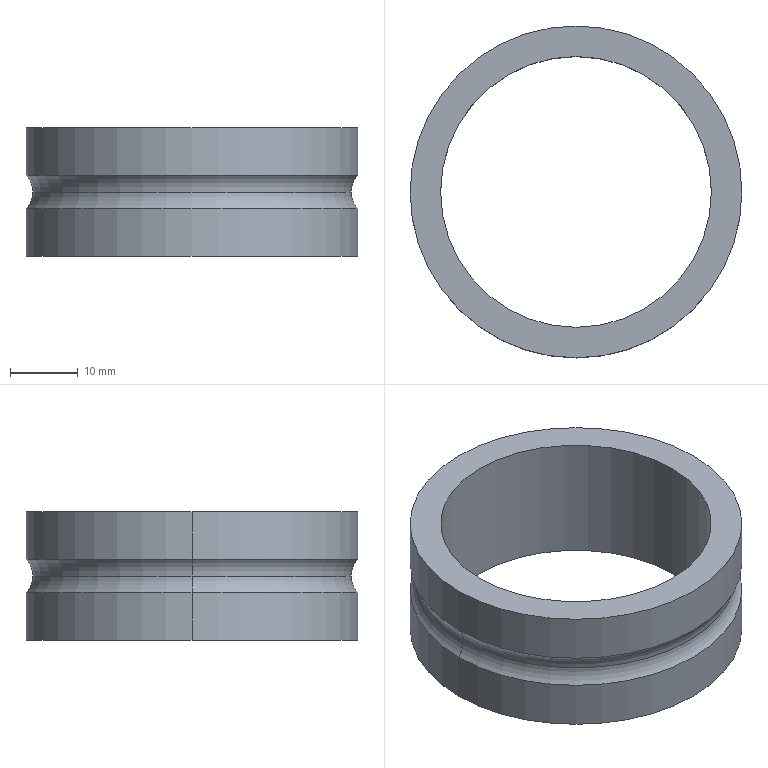Part | SolidWorks | 1 solid | 12 faces | box 49 x 49 x 19 mm | volume 11442 mm3 | cylinder 6 | torus 4 | plane 2 | commonest cylinder face diameters 49 x4 40 x2
STEP:
#1=CARTESIAN_POINT('',(-23.5,0.,-9.5));
#2=VERTEX_POINT('',#1);
#3=CARTESIAN_POINT('',(-24.5,0.,-11.949));
#4=VERTEX_POINT('',#3);
#5=CARTESIAN_POINT('',(-27.,0.,-9.5));
#6=DIRECTION('',(0.,1.,0.));
#7=DIRECTION('',(1.,0.,0.));
#8=AXIS2_PLACEMENT_3D('',#5,#6,#7);
#9=CIRCLE('',#8,3.5);
#10=EDGE_CURVE('',#2,#4,#9,.T.);
#11=ORIENTED_EDGE('',*,*,#10,.T.);
#12=CARTESIAN_POINT('',(24.5,0.,-11.949));
#13=VERTEX_POINT('',#12);
#14=CARTESIAN_POINT('',(0.,0.,-11.949));
#15=DIRECTION('',(0.,0.,-1.));
#16=DIRECTION('',(1.,0.,0.));
#17=AXIS2_PLACEMENT_3D('',#14,#15,#16);
#18=CIRCLE('',#17,24.5);
#19=EDGE_CURVE('',#13,#4,#18,.T.);
#20=ORIENTED_EDGE('',*,*,#19,.F.);
#21=CARTESIAN_POINT('',(23.5,0.,-9.5));
#22=VERTEX_POINT('',#21);
#23=CARTESIAN_POINT('',(27.,0.,-9.5));
#24=DIRECTION('',(0.,-1.,0.));
#25=DIRECTION('',(-1.,0.,0.));
#26=AXIS2_PLACEMENT_3D('',#23,#24,#25);
#27=CIRCLE('',#26,3.5);
#28=EDGE_CURVE('',#22,#13,#27,.T.);
#29=ORIENTED_EDGE('',*,*,#28,.F.);
#30=CARTESIAN_POINT('',(0.,0.,-9.5));
#31=DIRECTION('',(0.,0.,-1.));
#32=DIRECTION('',(1.,0.,0.));
#33=AXIS2_PLACEMENT_3D('',#30,#31,#32);
#34=CIRCLE('',#33,23.5);
#35=EDGE_CURVE('',#22,#2,#34,.T.);
#36=ORIENTED_EDGE('',*,*,#35,.T.);
#37=EDGE_LOOP('',(#11,#20,#29,#36));
#38=FACE_OUTER_BOUND('',#37,.T.);
#39=CARTESIAN_POINT('',(0.,0.,-9.5));
#40=DIRECTION('',(0.,0.,1.));
#41=DIRECTION('',(-1.,0.,0.));
#42=AXIS2_PLACEMENT_3D('',#39,#40,#41);
#43=TOROIDAL_SURFACE('',#42,27.,3.5);
#44=ADVANCED_FACE('',(#38),#43,.F.);
#45=ORIENTED_EDGE('',*,*,#28,.T.);
#46=CARTESIAN_POINT('',(0.,0.,-11.949));
#47=DIRECTION('',(0.,0.,-1.));
#48=DIRECTION('',(-1.,0.,0.));
#49=AXIS2_PLACEMENT_3D('',#46,#47,#48);
#50=CIRCLE('',#49,24.5);
#51=EDGE_CURVE('',#4,#13,#50,.T.);
#52=ORIENTED_EDGE('',*,*,#51,.F.);
#53=ORIENTED_EDGE('',*,*,#10,.F.);
#54=CARTESIAN_POINT('',(0.,0.,-9.5));
#55=DIRECTION('',(0.,0.,-1.));
#56=DIRECTION('',(-1.,0.,0.));
#57=AXIS2_PLACEMENT_3D('',#54,#55,#56);
#58=CIRCLE('',#57,23.5);
#59=EDGE_CURVE('',#2,#22,#58,.T.);
#60=ORIENTED_EDGE('',*,*,#59,.T.);
#61=EDGE_LOOP('',(#45,#52,#53,#60));
#62=FACE_OUTER_BOUND('',#61,.T.);
#63=CARTESIAN_POINT('',(0.,0.,-9.5));
#64=DIRECTION('',(0.,0.,1.));
#65=DIRECTION('',(1.,0.,0.));
#66=AXIS2_PLACEMENT_3D('',#63,#64,#65);
#67=TOROIDAL_SURFACE('',#66,27.,3.5);
#68=ADVANCED_FACE('',(#62),#67,.F.);
#69=CARTESIAN_POINT('',(-24.5,0.,0.));
#70=VERTEX_POINT('',#69);
#71=CARTESIAN_POINT('',(24.5,0.,0.));
#72=VERTEX_POINT('',#71);
#73=CARTESIAN_POINT('',(0.,0.,0.));
#74=DIRECTION('',(0.,0.,-1.));
#75=DIRECTION('',(-1.,0.,0.));
#76=AXIS2_PLACEMENT_3D('',#73,#74,#75);
#77=CIRCLE('',#76,24.5);
#78=EDGE_CURVE('',#70,#72,#77,.T.);
#79=ORIENTED_EDGE('',*,*,#78,.T.);
#80=CARTESIAN_POINT('',(24.5,0.,-7.051));
#81=VERTEX_POINT('',#80);
#82=CARTESIAN_POINT('',(24.5,0.,0.));
#83=DIRECTION('',(0.,0.,-1.));
#84=VECTOR('',#83,1000.);
#85=LINE('',#82,#84);
#86=EDGE_CURVE('',#72,#81,#85,.T.);
#87=ORIENTED_EDGE('',*,*,#86,.T.);
#88=CARTESIAN_POINT('',(-24.5,0.,-7.051));
#89=VERTEX_POINT('',#88);
#90=CARTESIAN_POINT('',(0.,0.,-7.051));
#91=DIRECTION('',(0.,0.,1.));
#92=DIRECTION('',(1.,0.,0.));
#93=AXIS2_PLACEMENT_3D('',#90,#91,#92);
#94=CIRCLE('',#93,24.5);
#95=EDGE_CURVE('',#81,#89,#94,.T.);
#96=ORIENTED_EDGE('',*,*,#95,.T.);
#97=CARTESIAN_POINT('',(-24.5,0.,0.));
#98=DIRECTION('',(0.,0.,-1.));
#99=VECTOR('',#98,1000.);
#100=LINE('',#97,#99);
#101=EDGE_CURVE('',#70,#89,#100,.T.);
#102=ORIENTED_EDGE('',*,*,#101,.F.);
#103=EDGE_LOOP('',(#79,#87,#96,#102));
#104=FACE_OUTER_BOUND('',#103,.T.);
#105=CARTESIAN_POINT('',(0.,0.,0.));
#106=DIRECTION('',(0.,0.,1.));
#107=DIRECTION('',(1.,0.,0.));
#108=AXIS2_PLACEMENT_3D('',#105,#106,#107);
#109=CYLINDRICAL_SURFACE('',#108,24.5);
#110=ADVANCED_FACE('',(#104),#109,.T.);
#111=ORIENTED_EDGE('',*,*,#59,.F.);
#112=CARTESIAN_POINT('',(-27.,0.,-9.5));
#113=DIRECTION('',(0.,1.,0.));
#114=DIRECTION('',(0.7143,0.,0.6999));
#115=AXIS2_PLACEMENT_3D('',#112,#113,#114);
#116=CIRCLE('',#115,3.5);
#117=EDGE_CURVE('',#89,#2,#116,.T.);
#118=ORIENTED_EDGE('',*,*,#117,.F.);
#119=ORIENTED_EDGE('',*,*,#95,.F.);
#120=CARTESIAN_POINT('',(27.,0.,-9.5));
#121=DIRECTION('',(0.,-1.,0.));
#122=DIRECTION('',(-0.7143,0.,0.6999));
#123=AXIS2_PLACEMENT_3D('',#120,#121,#122);
#124=CIRCLE('',#123,3.5);
#125=EDGE_CURVE('',#81,#22,#124,.T.);
#126=ORIENTED_EDGE('',*,*,#125,.T.);
#127=EDGE_LOOP('',(#111,#118,#119,#126));
#128=FACE_OUTER_BOUND('',#127,.T.);
#129=CARTESIAN_POINT('',(0.,0.,-9.5));
#130=DIRECTION('',(0.,0.,1.));
#131=DIRECTION('',(1.,0.,0.));
#132=AXIS2_PLACEMENT_3D('',#129,#130,#131);
#133=TOROIDAL_SURFACE('',#132,27.,3.5);
#134=ADVANCED_FACE('',(#128),#133,.F.);
#135=ORIENTED_EDGE('',*,*,#35,.F.);
#136=ORIENTED_EDGE('',*,*,#125,.F.);
#137=CARTESIAN_POINT('',(0.,0.,-7.051));
#138=DIRECTION('',(0.,0.,1.));
#139=DIRECTION('',(-1.,0.,0.));
#140=AXIS2_PLACEMENT_3D('',#137,#138,#139);
#141=CIRCLE('',#140,24.5);
#142=EDGE_CURVE('',#89,#81,#141,.T.);
#143=ORIENTED_EDGE('',*,*,#142,.F.);
#144=ORIENTED_EDGE('',*,*,#117,.T.);
#145=EDGE_LOOP('',(#135,#136,#143,#144));
#146=FACE_OUTER_BOUND('',#145,.T.);
#147=CARTESIAN_POINT('',(0.,0.,-9.5));
#148=DIRECTION('',(0.,0.,1.));
#149=DIRECTION('',(-1.,0.,0.));
#150=AXIS2_PLACEMENT_3D('',#147,#148,#149);
#151=TOROIDAL_SURFACE('',#150,27.,3.5);
#152=ADVANCED_FACE('',(#146),#151,.F.);
#153=ORIENTED_EDGE('',*,*,#86,.F.);
#154=CARTESIAN_POINT('',(0.,0.,0.));
#155=DIRECTION('',(0.,0.,-1.));
#156=DIRECTION('',(1.,0.,0.));
#157=AXIS2_PLACEMENT_3D('',#154,#155,#156);
#158=CIRCLE('',#157,24.5);
#159=EDGE_CURVE('',#72,#70,#158,.T.);
#160=ORIENTED_EDGE('',*,*,#159,.T.);
#161=ORIENTED_EDGE('',*,*,#101,.T.);
#162=ORIENTED_EDGE('',*,*,#142,.T.);
#163=EDGE_LOOP('',(#153,#160,#161,#162));
#164=FACE_OUTER_BOUND('',#163,.T.);
#165=CARTESIAN_POINT('',(0.,0.,0.));
#166=DIRECTION('',(0.,0.,1.));
#167=DIRECTION('',(1.,0.,0.));
#168=AXIS2_PLACEMENT_3D('',#165,#166,#167);
#169=CYLINDRICAL_SURFACE('',#168,24.5);
#170=ADVANCED_FACE('',(#164),#169,.T.);
#171=CARTESIAN_POINT('',(-20.,0.,0.));
#172=VERTEX_POINT('',#171);
#173=CARTESIAN_POINT('',(20.,0.,0.));
#174=VERTEX_POINT('',#173);
#175=CARTESIAN_POINT('',(0.,0.,0.));
#176=DIRECTION('',(0.,0.,1.));
#177=DIRECTION('',(-1.,0.,0.));
#178=AXIS2_PLACEMENT_3D('',#175,#176,#177);
#179=CIRCLE('',#178,20.);
#180=EDGE_CURVE('',#172,#174,#179,.T.);
#181=ORIENTED_EDGE('',*,*,#180,.F.);
#182=CARTESIAN_POINT('',(0.,0.,0.));
#183=DIRECTION('',(0.,0.,1.));
#184=DIRECTION('',(1.,0.,0.));
#185=AXIS2_PLACEMENT_3D('',#182,#183,#184);
#186=CIRCLE('',#185,20.);
#187=EDGE_CURVE('',#174,#172,#186,.T.);
#188=ORIENTED_EDGE('',*,*,#187,.F.);
#189=EDGE_LOOP('',(#181,#188));
#190=FACE_BOUND('',#189,.T.);
#191=ORIENTED_EDGE('',*,*,#78,.F.);
#192=ORIENTED_EDGE('',*,*,#159,.F.);
#193=EDGE_LOOP('',(#191,#192));
#194=FACE_OUTER_BOUND('',#193,.T.);
#195=CARTESIAN_POINT('',(0.,-20.,0.));
#196=DIRECTION('',(0.,0.,1.));
#197=DIRECTION('',(1.,0.,0.));
#198=AXIS2_PLACEMENT_3D('',#195,#196,#197);
#199=PLANE('',#198);
#200=ADVANCED_FACE('',(#190,#194),#199,.T.);
#201=CARTESIAN_POINT('',(20.,0.,-19.));
#202=VERTEX_POINT('',#201);
#203=CARTESIAN_POINT('',(20.,0.,0.));
#204=DIRECTION('',(0.,0.,-1.));
#205=VECTOR('',#204,1000.);
#206=LINE('',#203,#205);
#207=EDGE_CURVE('',#174,#202,#206,.T.);
#208=ORIENTED_EDGE('',*,*,#207,.F.);
#209=ORIENTED_EDGE('',*,*,#187,.T.);
#210=CARTESIAN_POINT('',(-20.,0.,-19.));
#211=VERTEX_POINT('',#210);
#212=CARTESIAN_POINT('',(-20.,0.,0.));
#213=DIRECTION('',(0.,0.,-1.));
#214=VECTOR('',#213,1000.);
#215=LINE('',#212,#214);
#216=EDGE_CURVE('',#172,#211,#215,.T.);
#217=ORIENTED_EDGE('',*,*,#216,.T.);
#218=CARTESIAN_POINT('',(0.,0.,-19.));
#219=DIRECTION('',(0.,0.,-1.));
#220=DIRECTION('',(-1.,0.,0.));
#221=AXIS2_PLACEMENT_3D('',#218,#219,#220);
#222=CIRCLE('',#221,20.);
#223=EDGE_CURVE('',#211,#202,#222,.T.);
#224=ORIENTED_EDGE('',*,*,#223,.T.);
#225=EDGE_LOOP('',(#208,#209,#217,#224));
#226=FACE_OUTER_BOUND('',#225,.T.);
#227=CARTESIAN_POINT('',(0.,0.,0.));
#228=DIRECTION('',(0.,0.,1.));
#229=DIRECTION('',(1.,0.,0.));
#230=AXIS2_PLACEMENT_3D('',#227,#228,#229);
#231=CYLINDRICAL_SURFACE('',#230,20.);
#232=ADVANCED_FACE('',(#226),#231,.F.);
#233=ORIENTED_EDGE('',*,*,#180,.T.);
#234=ORIENTED_EDGE('',*,*,#207,.T.);
#235=CARTESIAN_POINT('',(0.,0.,-19.));
#236=DIRECTION('',(0.,0.,-1.));
#237=DIRECTION('',(1.,0.,0.));
#238=AXIS2_PLACEMENT_3D('',#235,#236,#237);
#239=CIRCLE('',#238,20.);
#240=EDGE_CURVE('',#202,#211,#239,.T.);
#241=ORIENTED_EDGE('',*,*,#240,.T.);
#242=ORIENTED_EDGE('',*,*,#216,.F.);
#243=EDGE_LOOP('',(#233,#234,#241,#242));
#244=FACE_OUTER_BOUND('',#243,.T.);
#245=CARTESIAN_POINT('',(0.,0.,0.));
#246=DIRECTION('',(0.,0.,1.));
#247=DIRECTION('',(1.,0.,0.));
#248=AXIS2_PLACEMENT_3D('',#245,#246,#247);
#249=CYLINDRICAL_SURFACE('',#248,20.);
#250=ADVANCED_FACE('',(#244),#249,.F.);
#251=ORIENTED_EDGE('',*,*,#223,.F.);
#252=ORIENTED_EDGE('',*,*,#240,.F.);
#253=EDGE_LOOP('',(#251,#252));
#254=FACE_BOUND('',#253,.T.);
#255=CARTESIAN_POINT('',(-24.5,0.,-19.));
#256=VERTEX_POINT('',#255);
#257=CARTESIAN_POINT('',(24.5,0.,-19.));
#258=VERTEX_POINT('',#257);
#259=CARTESIAN_POINT('',(0.,0.,-19.));
#260=DIRECTION('',(0.,0.,1.));
#261=DIRECTION('',(-1.,0.,0.));
#262=AXIS2_PLACEMENT_3D('',#259,#260,#261);
#263=CIRCLE('',#262,24.5);
#264=EDGE_CURVE('',#256,#258,#263,.T.);
#265=ORIENTED_EDGE('',*,*,#264,.F.);
#266=CARTESIAN_POINT('',(0.,0.,-19.));
#267=DIRECTION('',(0.,0.,1.));
#268=DIRECTION('',(1.,0.,0.));
#269=AXIS2_PLACEMENT_3D('',#266,#267,#268);
#270=CIRCLE('',#269,24.5);
#271=EDGE_CURVE('',#258,#256,#270,.T.);
#272=ORIENTED_EDGE('',*,*,#271,.F.);
#273=EDGE_LOOP('',(#265,#272));
#274=FACE_OUTER_BOUND('',#273,.T.);
#275=CARTESIAN_POINT('',(0.,-24.5,-19.));
#276=DIRECTION('',(0.,0.,-1.));
#277=DIRECTION('',(0.,-1.,0.));
#278=AXIS2_PLACEMENT_3D('',#275,#276,#277);
#279=PLANE('',#278);
#280=ADVANCED_FACE('',(#254,#274),#279,.T.);
#281=CARTESIAN_POINT('',(24.5,0.,-11.949));
#282=DIRECTION('',(0.,0.,-1.));
#283=VECTOR('',#282,1000.);
#284=LINE('',#281,#283);
#285=EDGE_CURVE('',#13,#258,#284,.T.);
#286=ORIENTED_EDGE('',*,*,#285,.F.);
#287=ORIENTED_EDGE('',*,*,#19,.T.);
#288=CARTESIAN_POINT('',(-24.5,0.,-11.949));
#289=DIRECTION('',(0.,0.,-1.));
#290=VECTOR('',#289,1000.);
#291=LINE('',#288,#290);
#292=EDGE_CURVE('',#4,#256,#291,.T.);
#293=ORIENTED_EDGE('',*,*,#292,.T.);
#294=ORIENTED_EDGE('',*,*,#264,.T.);
#295=EDGE_LOOP('',(#286,#287,#293,#294));
#296=FACE_OUTER_BOUND('',#295,.T.);
#297=CARTESIAN_POINT('',(0.,0.,0.));
#298=DIRECTION('',(0.,0.,1.));
#299=DIRECTION('',(1.,0.,0.));
#300=AXIS2_PLACEMENT_3D('',#297,#298,#299);
#301=CYLINDRICAL_SURFACE('',#300,24.5);
#302=ADVANCED_FACE('',(#296),#301,.T.);
#303=ORIENTED_EDGE('',*,*,#51,.T.);
#304=ORIENTED_EDGE('',*,*,#285,.T.);
#305=ORIENTED_EDGE('',*,*,#271,.T.);
#306=ORIENTED_EDGE('',*,*,#292,.F.);
#307=EDGE_LOOP('',(#303,#304,#305,#306));
#308=FACE_OUTER_BOUND('',#307,.T.);
#309=CARTESIAN_POINT('',(0.,0.,0.));
#310=DIRECTION('',(0.,0.,1.));
#311=DIRECTION('',(1.,0.,0.));
#312=AXIS2_PLACEMENT_3D('',#309,#310,#311);
#313=CYLINDRICAL_SURFACE('',#312,24.5);
#314=ADVANCED_FACE('',(#308),#313,.T.);
#315=CLOSED_SHELL('',(#44,#68,#110,#134,#152,#170,#200,#232,#250,#280,#302,#314));
#316=MANIFOLD_SOLID_BREP('',#315);
#317=CARTESIAN_POINT('',(0.,0.,0.));
#318=DIRECTION('',(0.,0.,1.));
#319=DIRECTION('',(1.,0.,0.));
#320=AXIS2_PLACEMENT_3D('',#317,#318,#319);
#321=(LENGTH_UNIT()NAMED_UNIT(*)SI_UNIT(.MILLI.,.METRE.));
#322=UNCERTAINTY_MEASURE_WITH_UNIT(LENGTH_MEASURE(0.00001),#321,'','');
#323=(NAMED_UNIT(*)PLANE_ANGLE_UNIT()SI_UNIT($,.RADIAN.));
#324=(NAMED_UNIT(*)SI_UNIT($,.STERADIAN.)SOLID_ANGLE_UNIT());
#325=(GEOMETRIC_REPRESENTATION_CONTEXT(3)GLOBAL_UNCERTAINTY_ASSIGNED_CONTEXT((#322))GLOBAL_UNIT_ASSIGNED_CONTEXT((#321,#323,#324))REPRESENTATION_CONTEXT('',''));
#326=ADVANCED_BREP_SHAPE_REPRESENTATION('',(#316,#320),#325);